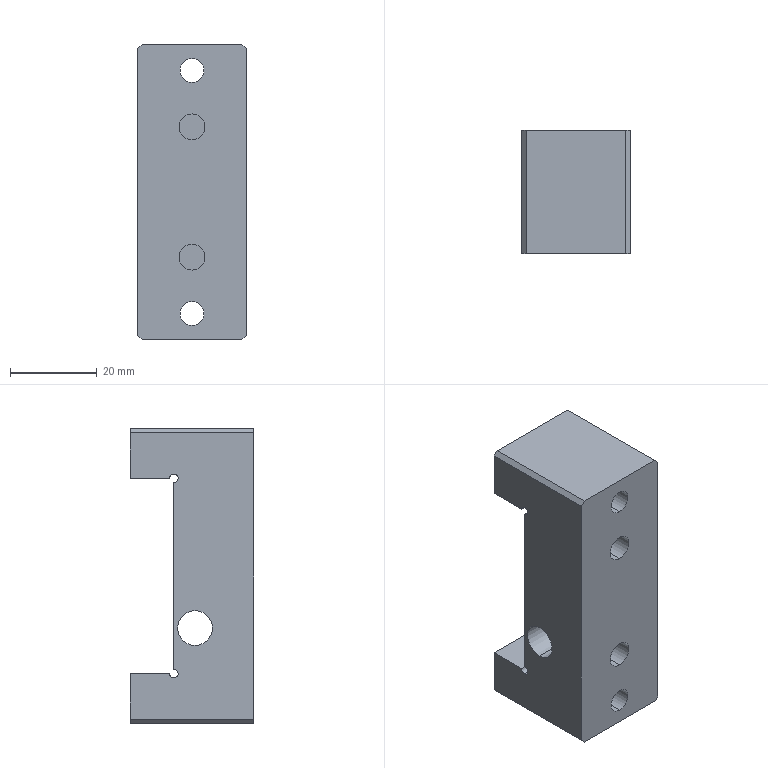Part | SolidWorks | features HoleWzd 3, ICE 2, Chamfer 1, Cut 1, Extrusion 1 | 1 solid | 51 faces | box 25 x 28.4 x 68 mm | volume 31309 mm3 | cylinder 25 | plane 18 | cone 8 | commonest cylinder face diameters 3.3 x8 5.5 x4 6 x4 10 x4 2 x3 8 x2